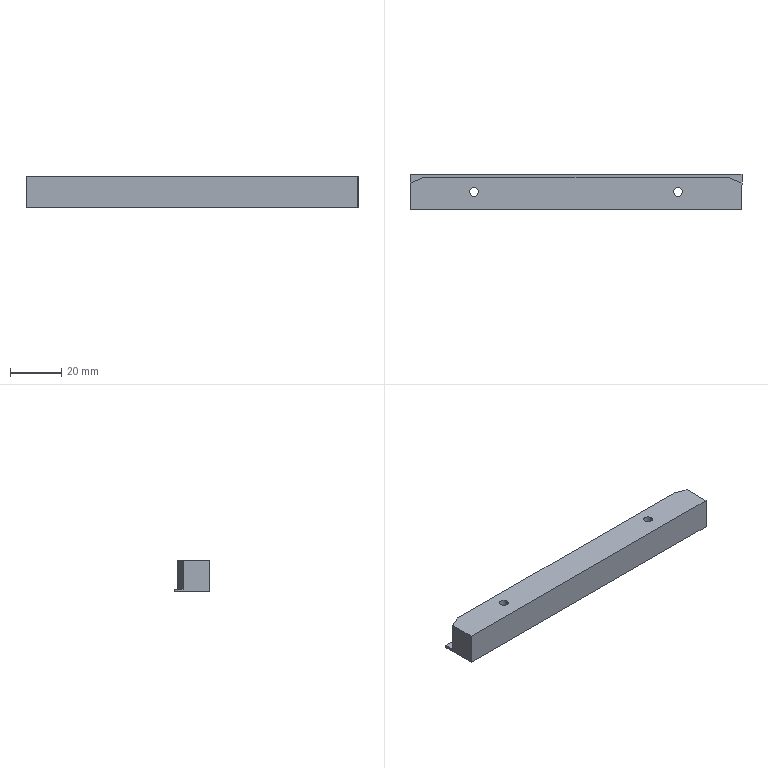Part | SolidWorks | features Chamfer 2, Extrusion 1, HoleWzd 1, ICE 1 | 1 solid | 20 faces | box 130 x 14 x 12.5 mm | volume 20035 mm3 | plane 12 | cylinder 8 | commonest cylinder face diameters 3.4 x4 6 x4
STEP:
#1=CARTESIAN_POINT('',(43.,0.,3.4));
#2=VERTEX_POINT('',#1);
#3=CARTESIAN_POINT('',(37.,0.,3.4));
#4=VERTEX_POINT('',#3);
#5=CARTESIAN_POINT('',(40.,0.,3.4));
#6=DIRECTION('',(0.,0.,-1.));
#7=DIRECTION('',(-1.,0.,0.));
#8=AXIS2_PLACEMENT_3D('',#5,#6,#7);
#9=CIRCLE('',#8,3.);
#10=EDGE_CURVE('',#2,#4,#9,.T.);
#11=ORIENTED_EDGE('',*,*,#10,.F.);
#12=CARTESIAN_POINT('',(43.,0.,0.));
#13=VERTEX_POINT('',#12);
#14=CARTESIAN_POINT('',(43.,0.,0.));
#15=DIRECTION('',(0.,0.,-1.));
#16=VECTOR('',#15,1000.);
#17=LINE('',#14,#16);
#18=EDGE_CURVE('',#2,#13,#17,.T.);
#19=ORIENTED_EDGE('',*,*,#18,.T.);
#20=CARTESIAN_POINT('',(37.,0.,0.));
#21=VERTEX_POINT('',#20);
#22=CARTESIAN_POINT('',(40.,0.,0.));
#23=DIRECTION('',(0.,0.,-1.));
#24=DIRECTION('',(-1.,0.,0.));
#25=AXIS2_PLACEMENT_3D('',#22,#23,#24);
#26=CIRCLE('',#25,3.);
#27=EDGE_CURVE('',#13,#21,#26,.T.);
#28=ORIENTED_EDGE('',*,*,#27,.T.);
#29=CARTESIAN_POINT('',(37.,0.,0.));
#30=DIRECTION('',(0.,0.,-1.));
#31=VECTOR('',#30,1000.);
#32=LINE('',#29,#31);
#33=EDGE_CURVE('',#4,#21,#32,.T.);
#34=ORIENTED_EDGE('',*,*,#33,.F.);
#35=EDGE_LOOP('',(#11,#19,#28,#34));
#36=FACE_OUTER_BOUND('',#35,.T.);
#37=CARTESIAN_POINT('',(40.,0.,0.));
#38=DIRECTION('',(0.,0.,-1.));
#39=DIRECTION('',(-1.,0.,0.));
#40=AXIS2_PLACEMENT_3D('',#37,#38,#39);
#41=CYLINDRICAL_SURFACE('',#40,3.);
#42=ADVANCED_FACE('',(#36),#41,.F.);
#43=CARTESIAN_POINT('',(41.7,0.,12.5));
#44=VERTEX_POINT('',#43);
#45=CARTESIAN_POINT('',(38.3,0.,12.5));
#46=VERTEX_POINT('',#45);
#47=CARTESIAN_POINT('',(40.,0.,12.5));
#48=DIRECTION('',(0.,0.,-1.));
#49=DIRECTION('',(-1.,0.,0.));
#50=AXIS2_PLACEMENT_3D('',#47,#48,#49);
#51=CIRCLE('',#50,1.7);
#52=EDGE_CURVE('',#44,#46,#51,.T.);
#53=ORIENTED_EDGE('',*,*,#52,.F.);
#54=CARTESIAN_POINT('',(41.7,0.,3.4));
#55=VERTEX_POINT('',#54);
#56=CARTESIAN_POINT('',(41.7,0.,0.));
#57=DIRECTION('',(0.,0.,-1.));
#58=VECTOR('',#57,1000.);
#59=LINE('',#56,#58);
#60=EDGE_CURVE('',#44,#55,#59,.T.);
#61=ORIENTED_EDGE('',*,*,#60,.T.);
#62=CARTESIAN_POINT('',(38.3,0.,3.4));
#63=VERTEX_POINT('',#62);
#64=CARTESIAN_POINT('',(40.,0.,3.4));
#65=DIRECTION('',(0.,0.,-1.));
#66=DIRECTION('',(-1.,0.,0.));
#67=AXIS2_PLACEMENT_3D('',#64,#65,#66);
#68=CIRCLE('',#67,1.7);
#69=EDGE_CURVE('',#55,#63,#68,.T.);
#70=ORIENTED_EDGE('',*,*,#69,.T.);
#71=CARTESIAN_POINT('',(38.3,0.,0.));
#72=DIRECTION('',(0.,0.,-1.));
#73=VECTOR('',#72,1000.);
#74=LINE('',#71,#73);
#75=EDGE_CURVE('',#46,#63,#74,.T.);
#76=ORIENTED_EDGE('',*,*,#75,.F.);
#77=EDGE_LOOP('',(#53,#61,#70,#76));
#78=FACE_OUTER_BOUND('',#77,.T.);
#79=CARTESIAN_POINT('',(40.,0.,0.));
#80=DIRECTION('',(0.,0.,-1.));
#81=DIRECTION('',(-1.,0.,0.));
#82=AXIS2_PLACEMENT_3D('',#79,#80,#81);
#83=CYLINDRICAL_SURFACE('',#82,1.7);
#84=ADVANCED_FACE('',(#78),#83,.F.);
#85=CARTESIAN_POINT('',(-37.,0.,3.4));
#86=VERTEX_POINT('',#85);
#87=CARTESIAN_POINT('',(-43.,0.,3.4));
#88=VERTEX_POINT('',#87);
#89=CARTESIAN_POINT('',(-40.,0.,3.4));
#90=DIRECTION('',(0.,0.,-1.));
#91=DIRECTION('',(-1.,0.,0.));
#92=AXIS2_PLACEMENT_3D('',#89,#90,#91);
#93=CIRCLE('',#92,3.);
#94=EDGE_CURVE('',#86,#88,#93,.T.);
#95=ORIENTED_EDGE('',*,*,#94,.F.);
#96=CARTESIAN_POINT('',(-37.,0.,0.));
#97=VERTEX_POINT('',#96);
#98=CARTESIAN_POINT('',(-37.,0.,0.));
#99=DIRECTION('',(0.,0.,-1.));
#100=VECTOR('',#99,1000.);
#101=LINE('',#98,#100);
#102=EDGE_CURVE('',#86,#97,#101,.T.);
#103=ORIENTED_EDGE('',*,*,#102,.T.);
#104=CARTESIAN_POINT('',(-43.,0.,0.));
#105=VERTEX_POINT('',#104);
#106=CARTESIAN_POINT('',(-40.,0.,0.));
#107=DIRECTION('',(0.,0.,-1.));
#108=DIRECTION('',(-1.,0.,0.));
#109=AXIS2_PLACEMENT_3D('',#106,#107,#108);
#110=CIRCLE('',#109,3.);
#111=EDGE_CURVE('',#97,#105,#110,.T.);
#112=ORIENTED_EDGE('',*,*,#111,.T.);
#113=CARTESIAN_POINT('',(-43.,0.,0.));
#114=DIRECTION('',(0.,0.,-1.));
#115=VECTOR('',#114,1000.);
#116=LINE('',#113,#115);
#117=EDGE_CURVE('',#88,#105,#116,.T.);
#118=ORIENTED_EDGE('',*,*,#117,.F.);
#119=EDGE_LOOP('',(#95,#103,#112,#118));
#120=FACE_OUTER_BOUND('',#119,.T.);
#121=CARTESIAN_POINT('',(-40.,0.,0.));
#122=DIRECTION('',(0.,0.,-1.));
#123=DIRECTION('',(-1.,0.,0.));
#124=AXIS2_PLACEMENT_3D('',#121,#122,#123);
#125=CYLINDRICAL_SURFACE('',#124,3.);
#126=ADVANCED_FACE('',(#120),#125,.F.);
#127=CARTESIAN_POINT('',(-38.3,0.,12.5));
#128=VERTEX_POINT('',#127);
#129=CARTESIAN_POINT('',(-41.7,0.,12.5));
#130=VERTEX_POINT('',#129);
#131=CARTESIAN_POINT('',(-40.,0.,12.5));
#132=DIRECTION('',(0.,0.,-1.));
#133=DIRECTION('',(-1.,0.,0.));
#134=AXIS2_PLACEMENT_3D('',#131,#132,#133);
#135=CIRCLE('',#134,1.7);
#136=EDGE_CURVE('',#128,#130,#135,.T.);
#137=ORIENTED_EDGE('',*,*,#136,.F.);
#138=CARTESIAN_POINT('',(-38.3,0.,3.4));
#139=VERTEX_POINT('',#138);
#140=CARTESIAN_POINT('',(-38.3,0.,0.));
#141=DIRECTION('',(0.,0.,-1.));
#142=VECTOR('',#141,1000.);
#143=LINE('',#140,#142);
#144=EDGE_CURVE('',#128,#139,#143,.T.);
#145=ORIENTED_EDGE('',*,*,#144,.T.);
#146=CARTESIAN_POINT('',(-41.7,0.,3.4));
#147=VERTEX_POINT('',#146);
#148=CARTESIAN_POINT('',(-40.,0.,3.4));
#149=DIRECTION('',(0.,0.,-1.));
#150=DIRECTION('',(-1.,0.,0.));
#151=AXIS2_PLACEMENT_3D('',#148,#149,#150);
#152=CIRCLE('',#151,1.7);
#153=EDGE_CURVE('',#139,#147,#152,.T.);
#154=ORIENTED_EDGE('',*,*,#153,.T.);
#155=CARTESIAN_POINT('',(-41.7,0.,0.));
#156=DIRECTION('',(0.,0.,-1.));
#157=VECTOR('',#156,1000.);
#158=LINE('',#155,#157);
#159=EDGE_CURVE('',#130,#147,#158,.T.);
#160=ORIENTED_EDGE('',*,*,#159,.F.);
#161=EDGE_LOOP('',(#137,#145,#154,#160));
#162=FACE_OUTER_BOUND('',#161,.T.);
#163=CARTESIAN_POINT('',(-40.,0.,0.));
#164=DIRECTION('',(0.,0.,-1.));
#165=DIRECTION('',(-1.,0.,0.));
#166=AXIS2_PLACEMENT_3D('',#163,#164,#165);
#167=CYLINDRICAL_SURFACE('',#166,1.7);
#168=ADVANCED_FACE('',(#162),#167,.F.);
#169=CARTESIAN_POINT('',(65.,3.5,1.));
#170=VERTEX_POINT('',#169);
#171=CARTESIAN_POINT('',(65.,7.,1.));
#172=VERTEX_POINT('',#171);
#173=CARTESIAN_POINT('',(65.,7.,1.));
#174=DIRECTION('',(0.,1.,0.));
#175=VECTOR('',#174,1000.);
#176=LINE('',#173,#175);
#177=EDGE_CURVE('',#170,#172,#176,.T.);
#178=ORIENTED_EDGE('',*,*,#177,.F.);
#179=CARTESIAN_POINT('',(65.,3.5,12.5));
#180=VERTEX_POINT('',#179);
#181=CARTESIAN_POINT('',(65.,3.5,12.5));
#182=DIRECTION('',(0.,0.,1.));
#183=VECTOR('',#182,1000.);
#184=LINE('',#181,#183);
#185=EDGE_CURVE('',#170,#180,#184,.T.);
#186=ORIENTED_EDGE('',*,*,#185,.T.);
#187=CARTESIAN_POINT('',(65.,-7.,12.5));
#188=VERTEX_POINT('',#187);
#189=CARTESIAN_POINT('',(65.,7.,12.5));
#190=DIRECTION('',(0.,1.,0.));
#191=VECTOR('',#190,1000.);
#192=LINE('',#189,#191);
#193=EDGE_CURVE('',#188,#180,#192,.T.);
#194=ORIENTED_EDGE('',*,*,#193,.F.);
#195=CARTESIAN_POINT('',(65.,-7.,0.));
#196=VERTEX_POINT('',#195);
#197=CARTESIAN_POINT('',(65.,-7.,12.5));
#198=DIRECTION('',(0.,0.,-1.));
#199=VECTOR('',#198,1000.);
#200=LINE('',#197,#199);
#201=EDGE_CURVE('',#188,#196,#200,.T.);
#202=ORIENTED_EDGE('',*,*,#201,.T.);
#203=CARTESIAN_POINT('',(65.,7.,0.));
#204=VERTEX_POINT('',#203);
#205=CARTESIAN_POINT('',(65.,7.,0.));
#206=DIRECTION('',(0.,1.,0.));
#207=VECTOR('',#206,1000.);
#208=LINE('',#205,#207);
#209=EDGE_CURVE('',#196,#204,#208,.T.);
#210=ORIENTED_EDGE('',*,*,#209,.T.);
#211=CARTESIAN_POINT('',(65.,7.,12.5));
#212=DIRECTION('',(0.,0.,-1.));
#213=VECTOR('',#212,1000.);
#214=LINE('',#211,#213);
#215=EDGE_CURVE('',#172,#204,#214,.T.);
#216=ORIENTED_EDGE('',*,*,#215,.F.);
#217=EDGE_LOOP('',(#178,#186,#194,#202,#210,#216));
#218=FACE_OUTER_BOUND('',#217,.T.);
#219=CARTESIAN_POINT('',(65.,7.,12.5));
#220=DIRECTION('',(-1.,0.,0.));
#221=DIRECTION('',(0.,0.,1.));
#222=AXIS2_PLACEMENT_3D('',#219,#220,#221);
#223=PLANE('',#222);
#224=ADVANCED_FACE('',(#218),#223,.F.);
#225=CARTESIAN_POINT('',(-65.,7.,1.));
#226=VERTEX_POINT('',#225);
#227=CARTESIAN_POINT('',(-65.,7.,0.));
#228=VERTEX_POINT('',#227);
#229=CARTESIAN_POINT('',(-65.,7.,12.5));
#230=DIRECTION('',(0.,0.,-1.));
#231=VECTOR('',#230,1000.);
#232=LINE('',#229,#231);
#233=EDGE_CURVE('',#226,#228,#232,.T.);
#234=ORIENTED_EDGE('',*,*,#233,.F.);
#235=CARTESIAN_POINT('',(-65.,7.,1.));
#236=DIRECTION('',(1.,0.,0.));
#237=VECTOR('',#236,1000.);
#238=LINE('',#235,#237);
#239=EDGE_CURVE('',#226,#172,#238,.T.);
#240=ORIENTED_EDGE('',*,*,#239,.T.);
#241=ORIENTED_EDGE('',*,*,#215,.T.);
#242=CARTESIAN_POINT('',(-65.,7.,0.));
#243=DIRECTION('',(-1.,0.,0.));
#244=VECTOR('',#243,1000.);
#245=LINE('',#242,#244);
#246=EDGE_CURVE('',#204,#228,#245,.T.);
#247=ORIENTED_EDGE('',*,*,#246,.T.);
#248=EDGE_LOOP('',(#234,#240,#241,#247));
#249=FACE_OUTER_BOUND('',#248,.T.);
#250=CARTESIAN_POINT('',(-65.,7.,12.5));
#251=DIRECTION('',(0.,-1.,0.));
#252=DIRECTION('',(0.,0.,-1.));
#253=AXIS2_PLACEMENT_3D('',#250,#251,#252);
#254=PLANE('',#253);
#255=ADVANCED_FACE('',(#249),#254,.F.);
#256=CARTESIAN_POINT('',(-65.,3.5,12.5));
#257=VERTEX_POINT('',#256);
#258=CARTESIAN_POINT('',(-65.,-7.,12.5));
#259=VERTEX_POINT('',#258);
#260=CARTESIAN_POINT('',(-65.,7.,12.5));
#261=DIRECTION('',(0.,-1.,0.));
#262=VECTOR('',#261,1000.);
#263=LINE('',#260,#262);
#264=EDGE_CURVE('',#257,#259,#263,.T.);
#265=ORIENTED_EDGE('',*,*,#264,.F.);
#266=CARTESIAN_POINT('',(-65.,3.5,1.));
#267=VERTEX_POINT('',#266);
#268=CARTESIAN_POINT('',(-65.,3.5,12.5));
#269=DIRECTION('',(0.,0.,-1.));
#270=VECTOR('',#269,1000.);
#271=LINE('',#268,#270);
#272=EDGE_CURVE('',#257,#267,#271,.T.);
#273=ORIENTED_EDGE('',*,*,#272,.T.);
#274=CARTESIAN_POINT('',(-65.,7.,1.));
#275=DIRECTION('',(0.,1.,0.));
#276=VECTOR('',#275,1000.);
#277=LINE('',#274,#276);
#278=EDGE_CURVE('',#267,#226,#277,.T.);
#279=ORIENTED_EDGE('',*,*,#278,.T.);
#280=ORIENTED_EDGE('',*,*,#233,.T.);
#281=CARTESIAN_POINT('',(-65.,-7.,0.));
#282=VERTEX_POINT('',#281);
#283=CARTESIAN_POINT('',(-65.,7.,0.));
#284=DIRECTION('',(0.,-1.,0.));
#285=VECTOR('',#284,1000.);
#286=LINE('',#283,#285);
#287=EDGE_CURVE('',#228,#282,#286,.T.);
#288=ORIENTED_EDGE('',*,*,#287,.T.);
#289=CARTESIAN_POINT('',(-65.,-7.,12.5));
#290=DIRECTION('',(0.,0.,-1.));
#291=VECTOR('',#290,1000.);
#292=LINE('',#289,#291);
#293=EDGE_CURVE('',#259,#282,#292,.T.);
#294=ORIENTED_EDGE('',*,*,#293,.F.);
#295=EDGE_LOOP('',(#265,#273,#279,#280,#288,#294));
#296=FACE_OUTER_BOUND('',#295,.T.);
#297=CARTESIAN_POINT('',(-65.,7.,12.5));
#298=DIRECTION('',(1.,0.,0.));
#299=DIRECTION('',(0.,0.,-1.));
#300=AXIS2_PLACEMENT_3D('',#297,#298,#299);
#301=PLANE('',#300);
#302=ADVANCED_FACE('',(#296),#301,.F.);
#303=CARTESIAN_POINT('',(-65.,-7.,0.));
#304=DIRECTION('',(1.,0.,0.));
#305=VECTOR('',#304,1000.);
#306=LINE('',#303,#305);
#307=EDGE_CURVE('',#282,#196,#306,.T.);
#308=ORIENTED_EDGE('',*,*,#307,.T.);
#309=ORIENTED_EDGE('',*,*,#201,.F.);
#310=CARTESIAN_POINT('',(-65.,-7.,12.5));
#311=DIRECTION('',(1.,0.,0.));
#312=VECTOR('',#311,1000.);
#313=LINE('',#310,#312);
#314=EDGE_CURVE('',#259,#188,#313,.T.);
#315=ORIENTED_EDGE('',*,*,#314,.F.);
#316=ORIENTED_EDGE('',*,*,#293,.T.);
#317=EDGE_LOOP('',(#308,#309,#315,#316));
#318=FACE_OUTER_BOUND('',#317,.T.);
#319=CARTESIAN_POINT('',(-65.,-7.,12.5));
#320=DIRECTION('',(0.,1.,0.));
#321=DIRECTION('',(0.,0.,1.));
#322=AXIS2_PLACEMENT_3D('',#319,#320,#321);
#323=PLANE('',#322);
#324=ADVANCED_FACE('',(#318),#323,.F.);
#325=CARTESIAN_POINT('',(40.,0.,12.5));
#326=DIRECTION('',(0.,0.,-1.));
#327=DIRECTION('',(-1.,0.,0.));
#328=AXIS2_PLACEMENT_3D('',#325,#326,#327);
#329=CIRCLE('',#328,1.7);
#330=EDGE_CURVE('',#46,#44,#329,.T.);
#331=ORIENTED_EDGE('',*,*,#330,.T.);
#332=ORIENTED_EDGE('',*,*,#52,.T.);
#333=EDGE_LOOP('',(#331,#332));
#334=FACE_BOUND('',#333,.T.);
#335=CARTESIAN_POINT('',(-40.,0.,12.5));
#336=DIRECTION('',(0.,0.,-1.));
#337=DIRECTION('',(-1.,0.,0.));
#338=AXIS2_PLACEMENT_3D('',#335,#336,#337);
#339=CIRCLE('',#338,1.7);
#340=EDGE_CURVE('',#130,#128,#339,.T.);
#341=ORIENTED_EDGE('',*,*,#340,.T.);
#342=ORIENTED_EDGE('',*,*,#136,.T.);
#343=EDGE_LOOP('',(#341,#342));
#344=FACE_BOUND('',#343,.T.);
#345=CARTESIAN_POINT('',(-60.,5.5,12.5));
#346=VERTEX_POINT('',#345);
#347=CARTESIAN_POINT('',(60.,5.5,12.5));
#348=VERTEX_POINT('',#347);
#349=CARTESIAN_POINT('',(-65.,5.5,12.5));
#350=DIRECTION('',(1.,0.,0.));
#351=VECTOR('',#350,1000.);
#352=LINE('',#349,#351);
#353=EDGE_CURVE('',#346,#348,#352,.T.);
#354=ORIENTED_EDGE('',*,*,#353,.F.);
#355=CARTESIAN_POINT('',(-10.172,25.431,12.5));
#356=DIRECTION('',(-0.9285,-0.3714,0.));
#357=VECTOR('',#356,1000.);
#358=LINE('',#355,#357);
#359=EDGE_CURVE('',#346,#257,#358,.T.);
#360=ORIENTED_EDGE('',*,*,#359,.T.);
#361=ORIENTED_EDGE('',*,*,#264,.T.);
#362=ORIENTED_EDGE('',*,*,#314,.T.);
#363=ORIENTED_EDGE('',*,*,#193,.T.);
#364=CARTESIAN_POINT('',(10.172,25.431,12.5));
#365=DIRECTION('',(-0.9285,0.3714,0.));
#366=VECTOR('',#365,1000.);
#367=LINE('',#364,#366);
#368=EDGE_CURVE('',#180,#348,#367,.T.);
#369=ORIENTED_EDGE('',*,*,#368,.T.);
#370=EDGE_LOOP('',(#354,#360,#361,#362,#363,#369));
#371=FACE_OUTER_BOUND('',#370,.T.);
#372=CARTESIAN_POINT('',(0.,0.,12.5));
#373=DIRECTION('',(0.,0.,1.));
#374=DIRECTION('',(1.,0.,0.));
#375=AXIS2_PLACEMENT_3D('',#372,#373,#374);
#376=PLANE('',#375);
#377=ADVANCED_FACE('',(#334,#344,#371),#376,.T.);
#378=CARTESIAN_POINT('',(40.,0.,0.));
#379=DIRECTION('',(0.,0.,-1.));
#380=DIRECTION('',(-1.,0.,0.));
#381=AXIS2_PLACEMENT_3D('',#378,#379,#380);
#382=CIRCLE('',#381,3.);
#383=EDGE_CURVE('',#21,#13,#382,.T.);
#384=ORIENTED_EDGE('',*,*,#383,.F.);
#385=ORIENTED_EDGE('',*,*,#27,.F.);
#386=EDGE_LOOP('',(#384,#385));
#387=FACE_BOUND('',#386,.T.);
#388=CARTESIAN_POINT('',(-40.,0.,0.));
#389=DIRECTION('',(0.,0.,-1.));
#390=DIRECTION('',(-1.,0.,0.));
#391=AXIS2_PLACEMENT_3D('',#388,#389,#390);
#392=CIRCLE('',#391,3.);
#393=EDGE_CURVE('',#105,#97,#392,.T.);
#394=ORIENTED_EDGE('',*,*,#393,.F.);
#395=ORIENTED_EDGE('',*,*,#111,.F.);
#396=EDGE_LOOP('',(#394,#395));
#397=FACE_BOUND('',#396,.T.);
#398=ORIENTED_EDGE('',*,*,#209,.F.);
#399=ORIENTED_EDGE('',*,*,#307,.F.);
#400=ORIENTED_EDGE('',*,*,#287,.F.);
#401=ORIENTED_EDGE('',*,*,#246,.F.);
#402=EDGE_LOOP('',(#398,#399,#400,#401));
#403=FACE_OUTER_BOUND('',#402,.T.);
#404=CARTESIAN_POINT('',(0.,0.,0.));
#405=DIRECTION('',(0.,0.,1.));
#406=DIRECTION('',(1.,0.,0.));
#407=AXIS2_PLACEMENT_3D('',#404,#405,#406);
#408=PLANE('',#407);
#409=ADVANCED_FACE('',(#387,#397,#403),#408,.F.);
#410=ORIENTED_EDGE('',*,*,#177,.T.);
#411=ORIENTED_EDGE('',*,*,#239,.F.);
#412=ORIENTED_EDGE('',*,*,#278,.F.);
#413=CARTESIAN_POINT('',(-60.,5.5,1.));
#414=VERTEX_POINT('',#413);
#415=CARTESIAN_POINT('',(-63.793,3.983,1.));
#416=DIRECTION('',(0.9285,0.3714,0.));
#417=VECTOR('',#416,1000.);
#418=LINE('',#415,#417);
#419=EDGE_CURVE('',#267,#414,#418,.T.);
#420=ORIENTED_EDGE('',*,*,#419,.T.);
#421=CARTESIAN_POINT('',(60.,5.5,1.));
#422=VERTEX_POINT('',#421);
#423=CARTESIAN_POINT('',(-65.,5.5,1.));
#424=DIRECTION('',(1.,0.,0.));
#425=VECTOR('',#424,1000.);
#426=LINE('',#423,#425);
#427=EDGE_CURVE('',#414,#422,#426,.T.);
#428=ORIENTED_EDGE('',*,*,#427,.T.);
#429=CARTESIAN_POINT('',(-48.276,48.81,1.));
#430=DIRECTION('',(0.9285,-0.3714,0.));
#431=VECTOR('',#430,1000.);
#432=LINE('',#429,#431);
#433=EDGE_CURVE('',#422,#170,#432,.T.);
#434=ORIENTED_EDGE('',*,*,#433,.T.);
#435=EDGE_LOOP('',(#410,#411,#412,#420,#428,#434));
#436=FACE_OUTER_BOUND('',#435,.T.);
#437=CARTESIAN_POINT('',(-65.,7.,1.));
#438=DIRECTION('',(0.,0.,-1.));
#439=DIRECTION('',(0.,1.,0.));
#440=AXIS2_PLACEMENT_3D('',#437,#438,#439);
#441=PLANE('',#440);
#442=ADVANCED_FACE('',(#436),#441,.F.);
#443=ORIENTED_EDGE('',*,*,#427,.F.);
#444=CARTESIAN_POINT('',(-60.,5.5,12.5));
#445=DIRECTION('',(0.,0.,1.));
#446=VECTOR('',#445,1000.);
#447=LINE('',#444,#446);
#448=EDGE_CURVE('',#414,#346,#447,.T.);
#449=ORIENTED_EDGE('',*,*,#448,.T.);
#450=ORIENTED_EDGE('',*,*,#353,.T.);
#451=CARTESIAN_POINT('',(60.,5.5,12.5));
#452=DIRECTION('',(0.,0.,-1.));
#453=VECTOR('',#452,1000.);
#454=LINE('',#451,#453);
#455=EDGE_CURVE('',#348,#422,#454,.T.);
#456=ORIENTED_EDGE('',*,*,#455,.T.);
#457=EDGE_LOOP('',(#443,#449,#450,#456));
#458=FACE_OUTER_BOUND('',#457,.T.);
#459=CARTESIAN_POINT('',(-65.,5.5,12.5));
#460=DIRECTION('',(0.,-1.,0.));
#461=DIRECTION('',(0.,0.,-1.));
#462=AXIS2_PLACEMENT_3D('',#459,#460,#461);
#463=PLANE('',#462);
#464=ADVANCED_FACE('',(#458),#463,.F.);
#465=ORIENTED_EDGE('',*,*,#368,.F.);
#466=ORIENTED_EDGE('',*,*,#185,.F.);
#467=ORIENTED_EDGE('',*,*,#433,.F.);
#468=ORIENTED_EDGE('',*,*,#455,.F.);
#469=EDGE_LOOP('',(#465,#466,#467,#468));
#470=FACE_OUTER_BOUND('',#469,.T.);
#471=CARTESIAN_POINT('',(60.,5.5,12.5));
#472=DIRECTION('',(-0.3714,-0.9285,0.));
#473=DIRECTION('',(0.,0.,-1.));
#474=AXIS2_PLACEMENT_3D('',#471,#472,#473);
#475=PLANE('',#474);
#476=ADVANCED_FACE('',(#470),#475,.F.);
#477=ORIENTED_EDGE('',*,*,#359,.F.);
#478=ORIENTED_EDGE('',*,*,#448,.F.);
#479=ORIENTED_EDGE('',*,*,#419,.F.);
#480=ORIENTED_EDGE('',*,*,#272,.F.);
#481=EDGE_LOOP('',(#477,#478,#479,#480));
#482=FACE_OUTER_BOUND('',#481,.T.);
#483=CARTESIAN_POINT('',(-65.,3.5,12.5));
#484=DIRECTION('',(0.3714,-0.9285,0.));
#485=DIRECTION('',(0.,0.,-1.));
#486=AXIS2_PLACEMENT_3D('',#483,#484,#485);
#487=PLANE('',#486);
#488=ADVANCED_FACE('',(#482),#487,.F.);
#489=ORIENTED_EDGE('',*,*,#144,.F.);
#490=ORIENTED_EDGE('',*,*,#340,.F.);
#491=ORIENTED_EDGE('',*,*,#159,.T.);
#492=CARTESIAN_POINT('',(-40.,0.,3.4));
#493=DIRECTION('',(0.,0.,-1.));
#494=DIRECTION('',(-1.,0.,0.));
#495=AXIS2_PLACEMENT_3D('',#492,#493,#494);
#496=CIRCLE('',#495,1.7);
#497=EDGE_CURVE('',#147,#139,#496,.T.);
#498=ORIENTED_EDGE('',*,*,#497,.T.);
#499=EDGE_LOOP('',(#489,#490,#491,#498));
#500=FACE_OUTER_BOUND('',#499,.T.);
#501=CARTESIAN_POINT('',(-40.,0.,0.));
#502=DIRECTION('',(0.,0.,-1.));
#503=DIRECTION('',(-1.,0.,0.));
#504=AXIS2_PLACEMENT_3D('',#501,#502,#503);
#505=CYLINDRICAL_SURFACE('',#504,1.7);
#506=ADVANCED_FACE('',(#500),#505,.F.);
#507=ORIENTED_EDGE('',*,*,#497,.F.);
#508=ORIENTED_EDGE('',*,*,#153,.F.);
#509=EDGE_LOOP('',(#507,#508));
#510=FACE_BOUND('',#509,.T.);
#511=CARTESIAN_POINT('',(-40.,0.,3.4));
#512=DIRECTION('',(0.,0.,-1.));
#513=DIRECTION('',(-1.,0.,0.));
#514=AXIS2_PLACEMENT_3D('',#511,#512,#513);
#515=CIRCLE('',#514,3.);
#516=EDGE_CURVE('',#88,#86,#515,.T.);
#517=ORIENTED_EDGE('',*,*,#516,.T.);
#518=ORIENTED_EDGE('',*,*,#94,.T.);
#519=EDGE_LOOP('',(#517,#518));
#520=FACE_OUTER_BOUND('',#519,.T.);
#521=CARTESIAN_POINT('',(-38.3,0.,3.4));
#522=DIRECTION('',(0.,0.,1.));
#523=DIRECTION('',(1.,0.,0.));
#524=AXIS2_PLACEMENT_3D('',#521,#522,#523);
#525=PLANE('',#524);
#526=ADVANCED_FACE('',(#510,#520),#525,.F.);
#527=ORIENTED_EDGE('',*,*,#102,.F.);
#528=ORIENTED_EDGE('',*,*,#516,.F.);
#529=ORIENTED_EDGE('',*,*,#117,.T.);
#530=ORIENTED_EDGE('',*,*,#393,.T.);
#531=EDGE_LOOP('',(#527,#528,#529,#530));
#532=FACE_OUTER_BOUND('',#531,.T.);
#533=CARTESIAN_POINT('',(-40.,0.,0.));
#534=DIRECTION('',(0.,0.,-1.));
#535=DIRECTION('',(-1.,0.,0.));
#536=AXIS2_PLACEMENT_3D('',#533,#534,#535);
#537=CYLINDRICAL_SURFACE('',#536,3.);
#538=ADVANCED_FACE('',(#532),#537,.F.);
#539=ORIENTED_EDGE('',*,*,#60,.F.);
#540=ORIENTED_EDGE('',*,*,#330,.F.);
#541=ORIENTED_EDGE('',*,*,#75,.T.);
#542=CARTESIAN_POINT('',(40.,0.,3.4));
#543=DIRECTION('',(0.,0.,-1.));
#544=DIRECTION('',(-1.,0.,0.));
#545=AXIS2_PLACEMENT_3D('',#542,#543,#544);
#546=CIRCLE('',#545,1.7);
#547=EDGE_CURVE('',#63,#55,#546,.T.);
#548=ORIENTED_EDGE('',*,*,#547,.T.);
#549=EDGE_LOOP('',(#539,#540,#541,#548));
#550=FACE_OUTER_BOUND('',#549,.T.);
#551=CARTESIAN_POINT('',(40.,0.,0.));
#552=DIRECTION('',(0.,0.,-1.));
#553=DIRECTION('',(-1.,0.,0.));
#554=AXIS2_PLACEMENT_3D('',#551,#552,#553);
#555=CYLINDRICAL_SURFACE('',#554,1.7);
#556=ADVANCED_FACE('',(#550),#555,.F.);
#557=ORIENTED_EDGE('',*,*,#547,.F.);
#558=ORIENTED_EDGE('',*,*,#69,.F.);
#559=EDGE_LOOP('',(#557,#558));
#560=FACE_BOUND('',#559,.T.);
#561=CARTESIAN_POINT('',(40.,0.,3.4));
#562=DIRECTION('',(0.,0.,-1.));
#563=DIRECTION('',(-1.,0.,0.));
#564=AXIS2_PLACEMENT_3D('',#561,#562,#563);
#565=CIRCLE('',#564,3.);
#566=EDGE_CURVE('',#4,#2,#565,.T.);
#567=ORIENTED_EDGE('',*,*,#566,.T.);
#568=ORIENTED_EDGE('',*,*,#10,.T.);
#569=EDGE_LOOP('',(#567,#568));
#570=FACE_OUTER_BOUND('',#569,.T.);
#571=CARTESIAN_POINT('',(41.7,0.,3.4));
#572=DIRECTION('',(0.,0.,1.));
#573=DIRECTION('',(1.,0.,0.));
#574=AXIS2_PLACEMENT_3D('',#571,#572,#573);
#575=PLANE('',#574);
#576=ADVANCED_FACE('',(#560,#570),#575,.F.);
#577=ORIENTED_EDGE('',*,*,#18,.F.);
#578=ORIENTED_EDGE('',*,*,#566,.F.);
#579=ORIENTED_EDGE('',*,*,#33,.T.);
#580=ORIENTED_EDGE('',*,*,#383,.T.);
#581=EDGE_LOOP('',(#577,#578,#579,#580));
#582=FACE_OUTER_BOUND('',#581,.T.);
#583=CARTESIAN_POINT('',(40.,0.,0.));
#584=DIRECTION('',(0.,0.,-1.));
#585=DIRECTION('',(-1.,0.,0.));
#586=AXIS2_PLACEMENT_3D('',#583,#584,#585);
#587=CYLINDRICAL_SURFACE('',#586,3.);
#588=ADVANCED_FACE('',(#582),#587,.F.);
#589=CLOSED_SHELL('',(#42,#84,#126,#168,#224,#255,#302,#324,#377,#409,#442,#464,#476,#488,#506,#526,#538,#556,#576,#588));
#590=MANIFOLD_SOLID_BREP('',#589);
#591=CARTESIAN_POINT('',(0.,0.,0.));
#592=DIRECTION('',(0.,0.,1.));
#593=DIRECTION('',(1.,0.,0.));
#594=AXIS2_PLACEMENT_3D('',#591,#592,#593);
#595=(LENGTH_UNIT()NAMED_UNIT(*)SI_UNIT(.MILLI.,.METRE.));
#596=UNCERTAINTY_MEASURE_WITH_UNIT(LENGTH_MEASURE(0.00001),#595,'','');
#597=(NAMED_UNIT(*)PLANE_ANGLE_UNIT()SI_UNIT($,.RADIAN.));
#598=(NAMED_UNIT(*)SI_UNIT($,.STERADIAN.)SOLID_ANGLE_UNIT());
#599=(GEOMETRIC_REPRESENTATION_CONTEXT(3)GLOBAL_UNCERTAINTY_ASSIGNED_CONTEXT((#596))GLOBAL_UNIT_ASSIGNED_CONTEXT((#595,#597,#598))REPRESENTATION_CONTEXT('',''));
#600=ADVANCED_BREP_SHAPE_REPRESENTATION('',(#590,#594),#599);